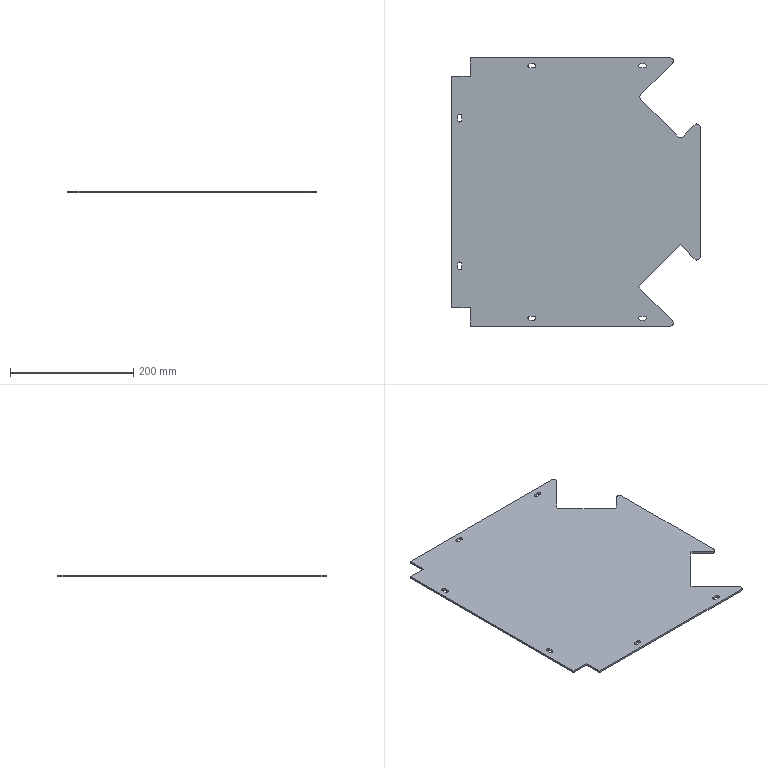Part | SolidWorks | features ICE 3, Cut 2, Extrusion 1, Fillet 1, MirrorPattern 1 | 1 solid | 52 faces | box 404 x 436 x 3 mm | volume 471052 mm3 | plane 28 | cylinder 24 | commonest cylinder face diameters 6.6 x16 10 x8